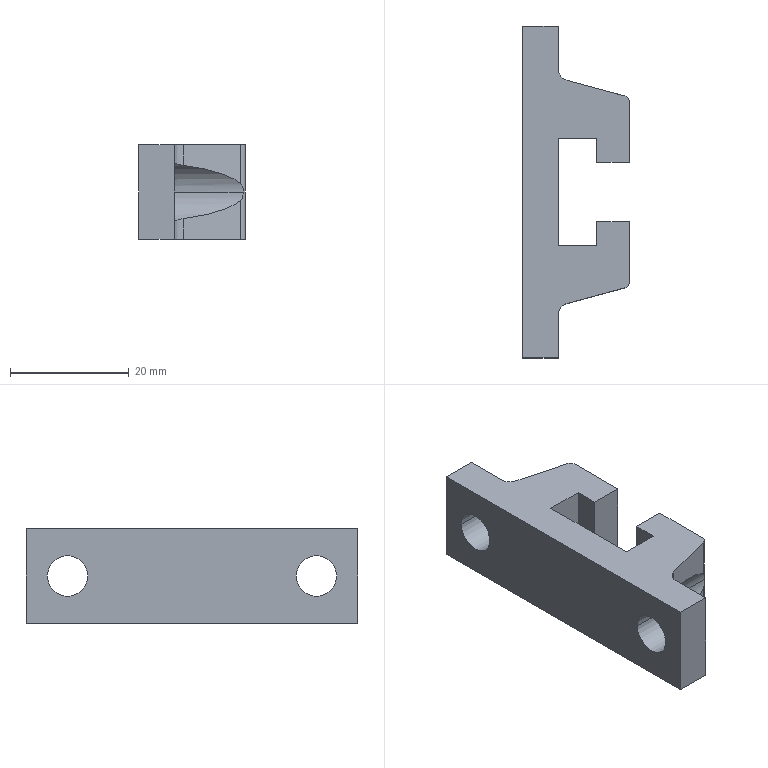Part | STEP file | _YA-03_CQ2.stp | 1 solid | 33 faces | box 18 x 56 x 16 mm | volume 8735 mm3 | plane 20 | cylinder 13 | commonest cylinder face diameters 4 x4 6.8 x4 10 x3 2 x2